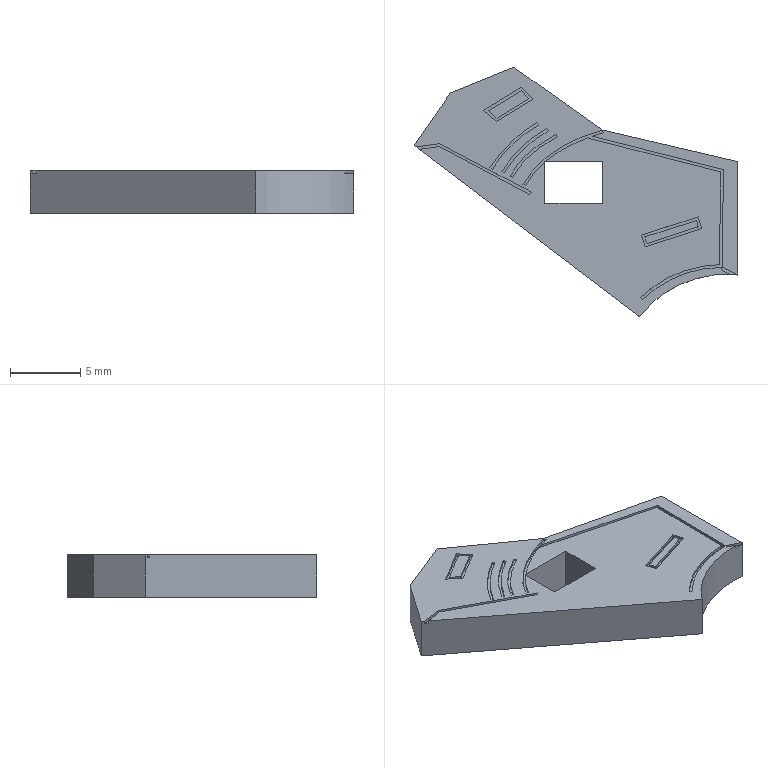Part | SolidWorks | features BaseBody 1 | 1 solid | 73 faces | box 23.095 x 17.792 x 3 mm | volume 604.555 mm3 | plane 59 | spline 12 | cylinder 2 | commonest cylinder face diameters 16.185 x1 16.585 x1